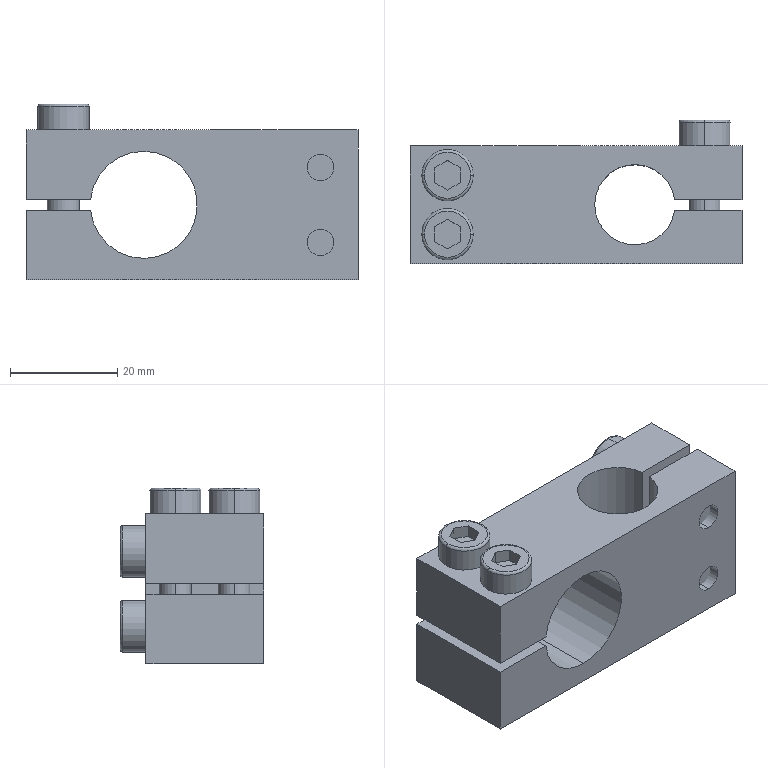Part | SolidWorks | features ICE 7, Fillet 2, MirrorSolid 2, MoveCopyBody 2, Revolution 2, Extrusion 1 | 5 solids | 97 faces | box 62 x 26.8 x 32.8 mm | volume 26392 mm3 | plane 52 | cylinder 37 | torus 8 | commonest cylinder face diameters 4.918 x8 6 x8 6.6 x8 9.6 x8 20 x3 15 x2